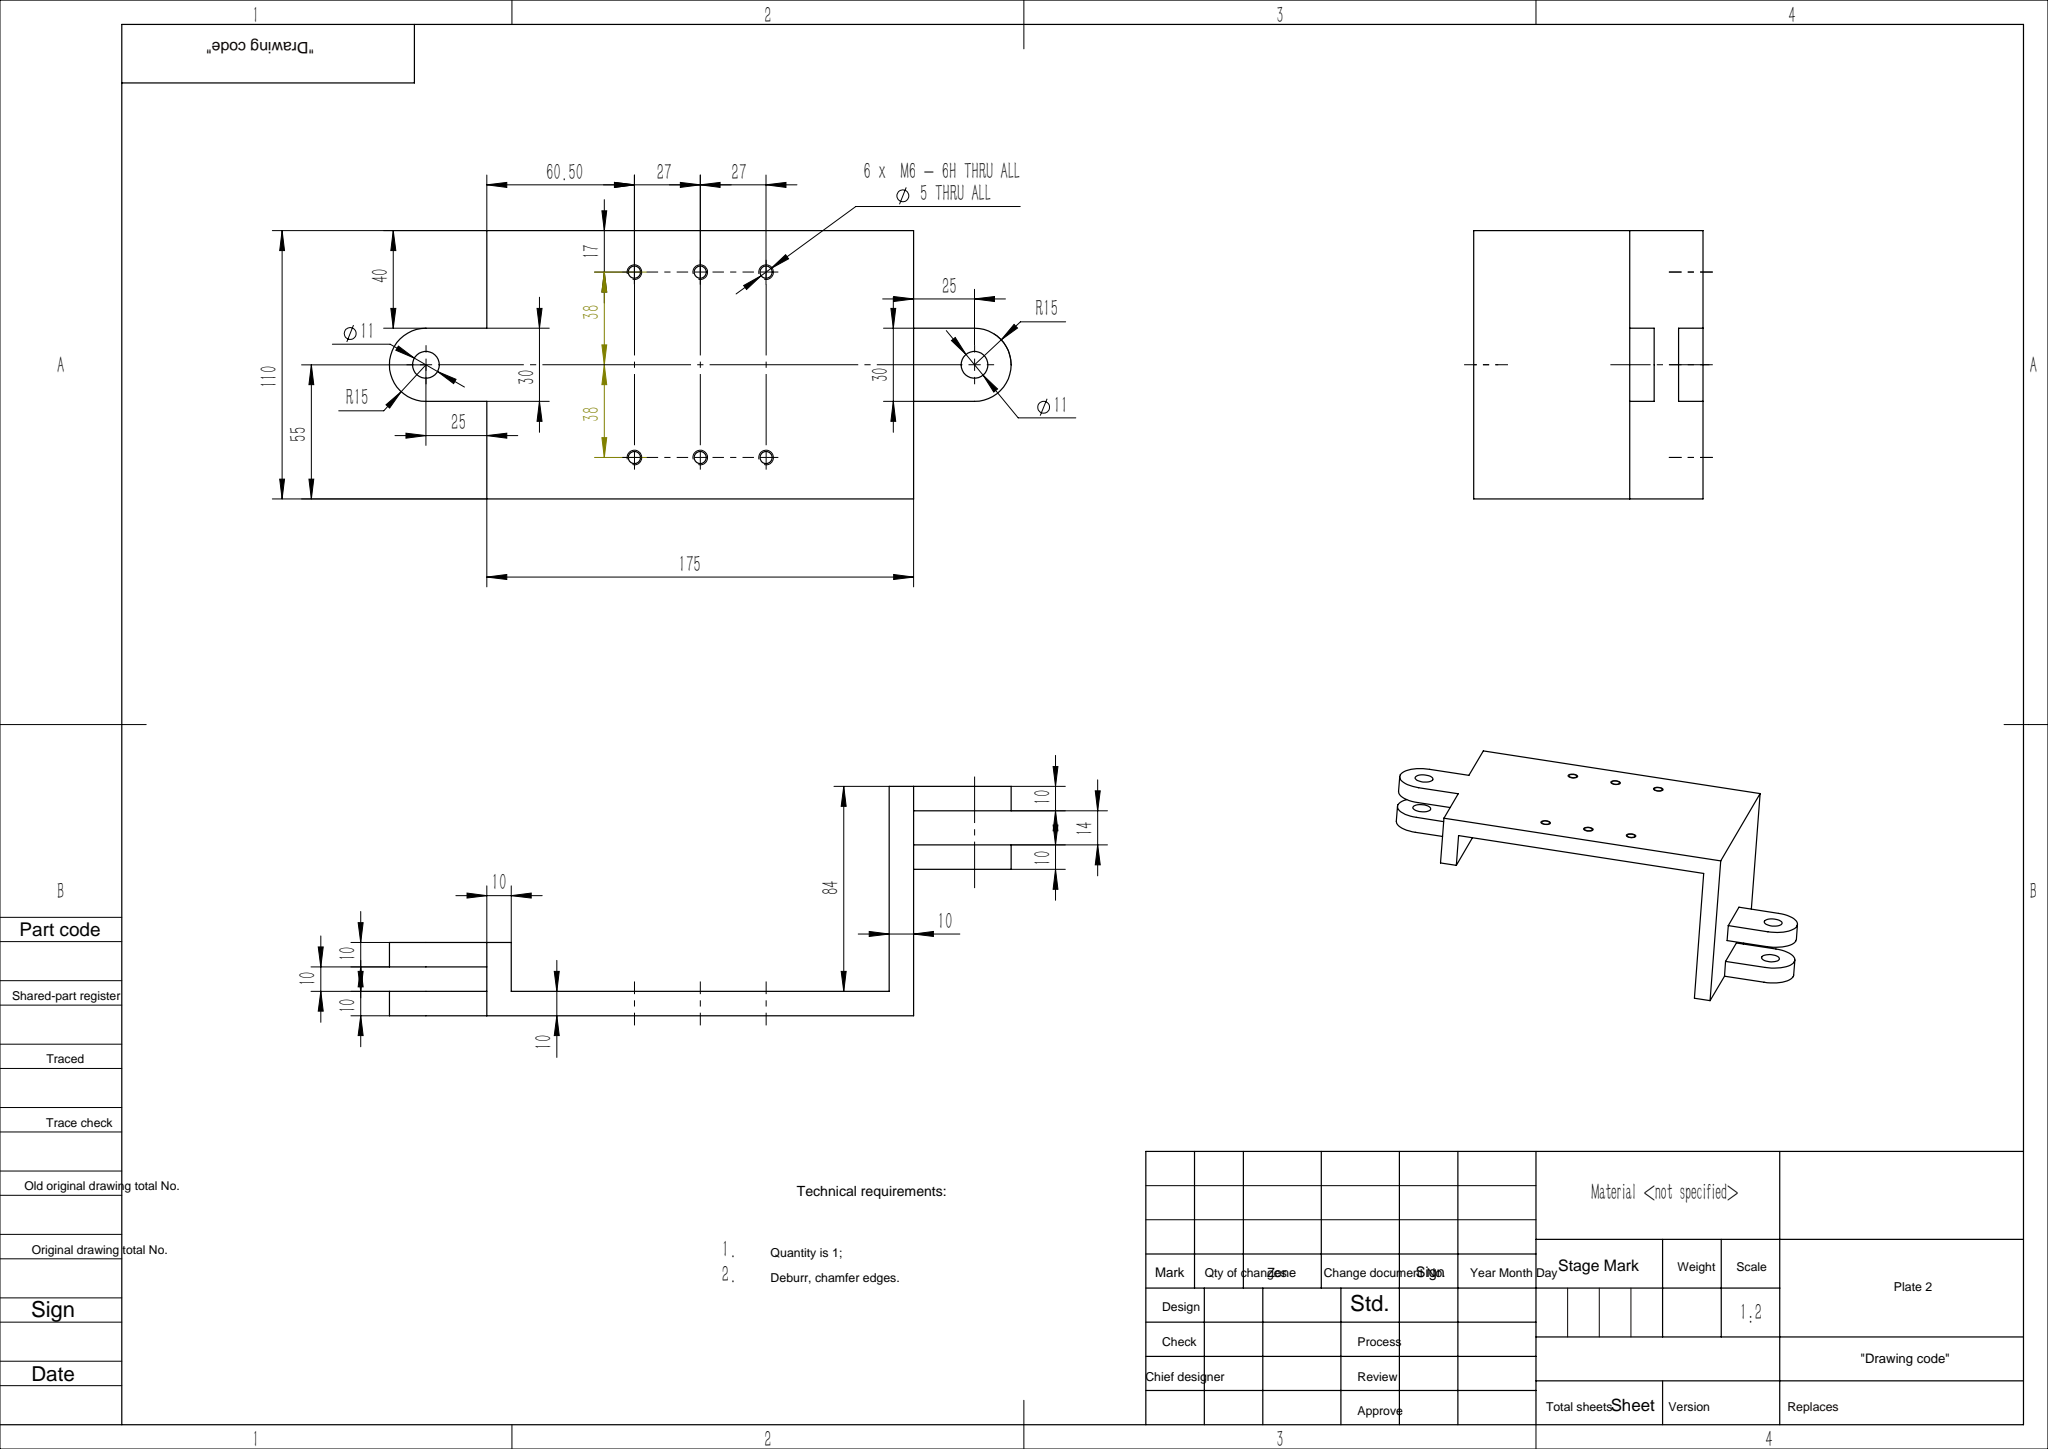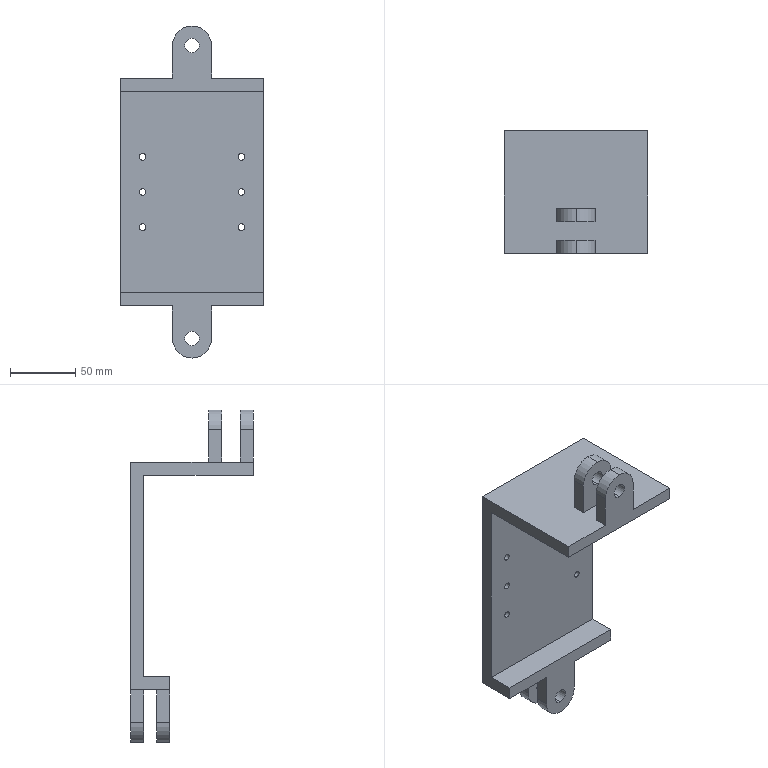Part | SolidWorks | features ICE 6, Fillet 2, LPattern 2, Extrusion 1, HoleWzd 1 | 1 solid | 51 faces | box 110 x 94 x 255 mm | volume 346058 mm3 | cylinder 28 | plane 23 | commonest cylinder face diameters 5 x12 11 x8 30 x8